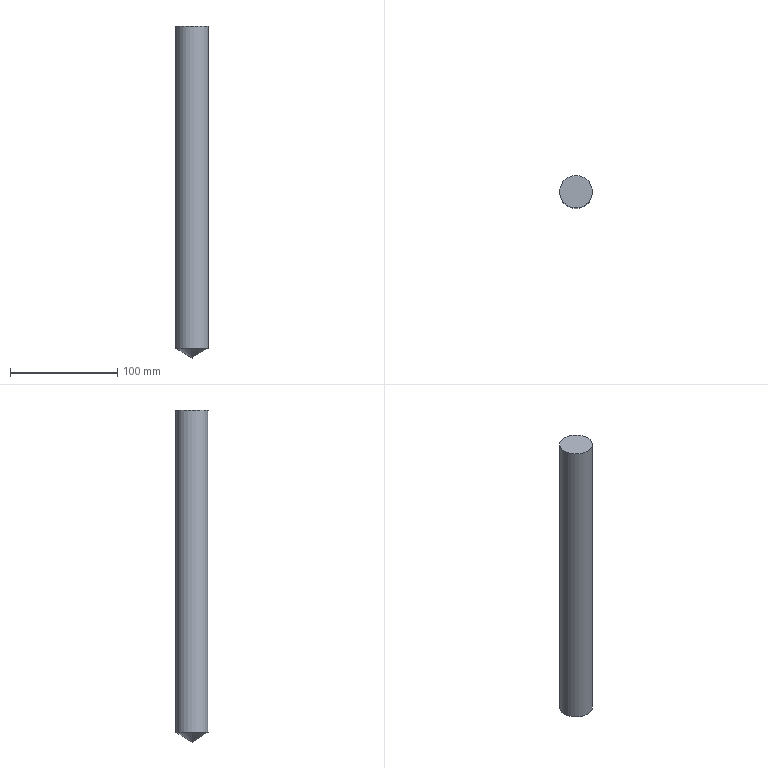Part | STEP file | solid 161 | 1 solid | 3 faces | box 30.5 x 30.5 x 309.163 mm | volume 221417 mm3 | cylinder 1 | plane 1 | cone 1 | commonest cylinder face diameters 30.5 x1